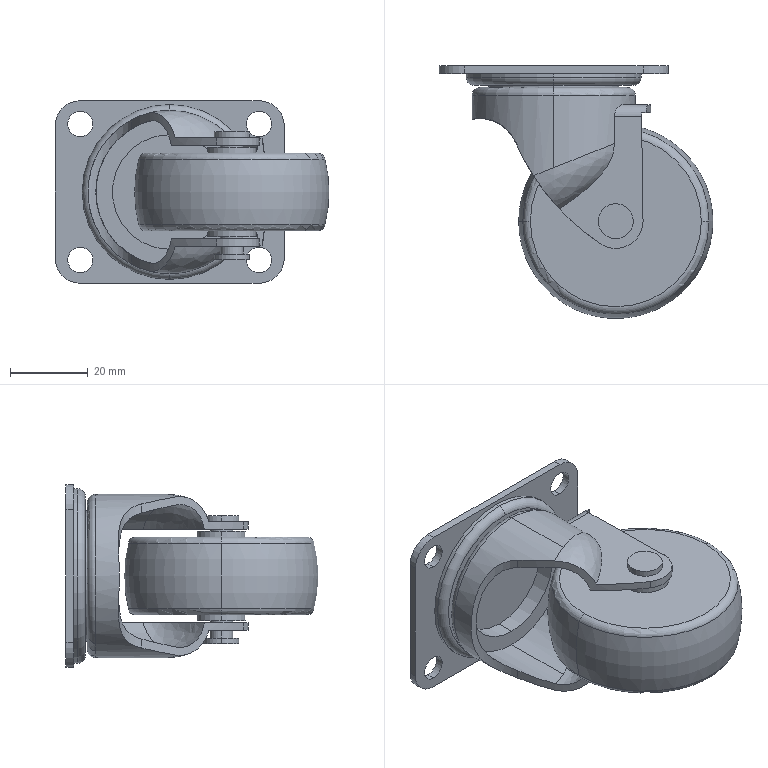Part | SolidWorks | features BaseBody 1 | 1 solid | 90 faces | box 70.5 x 65 x 47 mm | volume 52288 mm3 | cylinder 50 | plane 26 | torus 10 | spline 4 | commonest cylinder face diameters 6 x8 6.5 x8 9 x4 12.5 x4 13 x4 14 x4